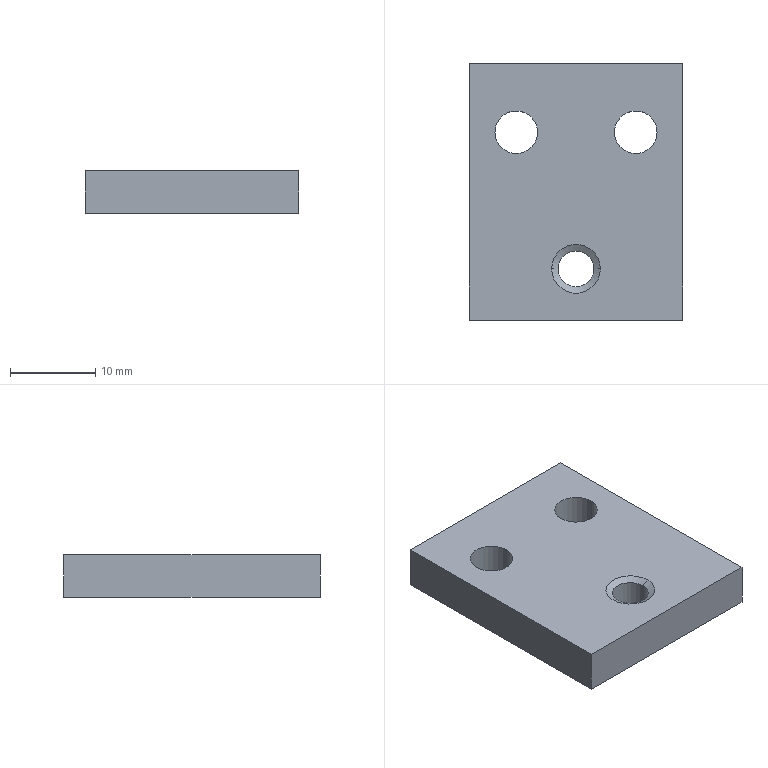Part | NX | 1 solid | 14 faces | box 25 x 30 x 5 mm | volume 3482 mm3 | plane 6 | cylinder 6 | cone 2 | commonest cylinder face diameters 5 x4 4.2 x2
STEP:
#1=CARTESIAN_POINT('',(-12.5,-9.53,2.5));
#2=VERTEX_POINT('',#1);
#3=CARTESIAN_POINT('',(-12.5,20.47,2.5));
#4=VERTEX_POINT('',#3);
#5=CARTESIAN_POINT('',(-12.5,0.,2.5));
#6=DIRECTION('',(0.,1.,0.));
#7=VECTOR('',#6,1000.);
#8=LINE('',#5,#7);
#9=EDGE_CURVE('',#2,#4,#8,.T.);
#10=ORIENTED_EDGE('',*,*,#9,.F.);
#11=CARTESIAN_POINT('',(12.5,-9.53,2.5));
#12=VERTEX_POINT('',#11);
#13=CARTESIAN_POINT('',(0.,-9.53,2.5));
#14=DIRECTION('',(-1.,0.,0.));
#15=VECTOR('',#14,1000.);
#16=LINE('',#13,#15);
#17=EDGE_CURVE('',#12,#2,#16,.T.);
#18=ORIENTED_EDGE('',*,*,#17,.F.);
#19=CARTESIAN_POINT('',(12.5,20.47,2.5));
#20=VERTEX_POINT('',#19);
#21=CARTESIAN_POINT('',(12.5,0.,2.5));
#22=DIRECTION('',(0.,1.,0.));
#23=VECTOR('',#22,1000.);
#24=LINE('',#21,#23);
#25=EDGE_CURVE('',#12,#20,#24,.T.);
#26=ORIENTED_EDGE('',*,*,#25,.T.);
#27=CARTESIAN_POINT('',(0.,20.47,2.5));
#28=DIRECTION('',(1.,0.,0.));
#29=VECTOR('',#28,1000.);
#30=LINE('',#27,#29);
#31=EDGE_CURVE('',#4,#20,#30,.T.);
#32=ORIENTED_EDGE('',*,*,#31,.F.);
#33=EDGE_LOOP('',(#10,#18,#26,#32));
#34=FACE_BOUND('',#33,.T.);
#35=CARTESIAN_POINT('',(-9.5,12.47,2.5));
#36=VERTEX_POINT('',#35);
#37=CARTESIAN_POINT('',(-4.5,12.47,2.5));
#38=VERTEX_POINT('',#37);
#39=CARTESIAN_POINT('',(-7.,12.47,2.5));
#40=DIRECTION('',(0.,0.,-1.));
#41=DIRECTION('',(-1.,0.,0.));
#42=AXIS2_PLACEMENT_3D('',#39,#40,#41);
#43=CIRCLE('',#42,2.5);
#44=EDGE_CURVE('',#36,#38,#43,.T.);
#45=ORIENTED_EDGE('',*,*,#44,.T.);
#46=CARTESIAN_POINT('',(-7.,12.47,2.5));
#47=DIRECTION('',(0.,0.,-1.));
#48=DIRECTION('',(-1.,0.,0.));
#49=AXIS2_PLACEMENT_3D('',#46,#47,#48);
#50=CIRCLE('',#49,2.5);
#51=EDGE_CURVE('',#38,#36,#50,.T.);
#52=ORIENTED_EDGE('',*,*,#51,.T.);
#53=EDGE_LOOP('',(#45,#52));
#54=FACE_BOUND('',#53,.T.);
#55=CARTESIAN_POINT('',(2.86,-3.53,2.5));
#56=VERTEX_POINT('',#55);
#57=CARTESIAN_POINT('',(-2.86,-3.53,2.5));
#58=VERTEX_POINT('',#57);
#59=CARTESIAN_POINT('',(0.,-3.53,2.5));
#60=DIRECTION('',(0.,0.,1.));
#61=DIRECTION('',(1.,0.,0.));
#62=AXIS2_PLACEMENT_3D('',#59,#60,#61);
#63=CIRCLE('',#62,2.86);
#64=EDGE_CURVE('',#56,#58,#63,.T.);
#65=ORIENTED_EDGE('',*,*,#64,.F.);
#66=CARTESIAN_POINT('',(0.,-3.53,2.5));
#67=DIRECTION('',(0.,0.,1.));
#68=DIRECTION('',(1.,0.,0.));
#69=AXIS2_PLACEMENT_3D('',#66,#67,#68);
#70=CIRCLE('',#69,2.86);
#71=EDGE_CURVE('',#58,#56,#70,.T.);
#72=ORIENTED_EDGE('',*,*,#71,.F.);
#73=EDGE_LOOP('',(#65,#72));
#74=FACE_BOUND('',#73,.T.);
#75=CARTESIAN_POINT('',(9.5,12.47,2.5));
#76=VERTEX_POINT('',#75);
#77=CARTESIAN_POINT('',(4.5,12.47,2.5));
#78=VERTEX_POINT('',#77);
#79=CARTESIAN_POINT('',(7.,12.47,2.5));
#80=DIRECTION('',(0.,0.,-1.));
#81=DIRECTION('',(-1.,0.,0.));
#82=AXIS2_PLACEMENT_3D('',#79,#80,#81);
#83=CIRCLE('',#82,2.5);
#84=EDGE_CURVE('',#76,#78,#83,.T.);
#85=ORIENTED_EDGE('',*,*,#84,.T.);
#86=CARTESIAN_POINT('',(7.,12.47,2.5));
#87=DIRECTION('',(0.,0.,-1.));
#88=DIRECTION('',(-1.,0.,0.));
#89=AXIS2_PLACEMENT_3D('',#86,#87,#88);
#90=CIRCLE('',#89,2.5);
#91=EDGE_CURVE('',#78,#76,#90,.T.);
#92=ORIENTED_EDGE('',*,*,#91,.T.);
#93=EDGE_LOOP('',(#85,#92));
#94=FACE_BOUND('',#93,.T.);
#95=CARTESIAN_POINT('',(0.,0.,2.5));
#96=DIRECTION('',(0.,0.,1.));
#97=DIRECTION('',(1.,0.,0.));
#98=AXIS2_PLACEMENT_3D('',#95,#96,#97);
#99=PLANE('',#98);
#100=ADVANCED_FACE('',(#34,#54,#74,#94),#99,.T.);
#101=CARTESIAN_POINT('',(-12.5,-9.53,-2.5));
#102=VERTEX_POINT('',#101);
#103=CARTESIAN_POINT('',(-12.5,20.47,-2.5));
#104=VERTEX_POINT('',#103);
#105=CARTESIAN_POINT('',(-12.5,0.,-2.5));
#106=DIRECTION('',(0.,1.,0.));
#107=VECTOR('',#106,1000.);
#108=LINE('',#105,#107);
#109=EDGE_CURVE('',#102,#104,#108,.T.);
#110=ORIENTED_EDGE('',*,*,#109,.F.);
#111=CARTESIAN_POINT('',(-12.5,-9.53,0.));
#112=DIRECTION('',(0.,0.,-1.));
#113=VECTOR('',#112,1000.);
#114=LINE('',#111,#113);
#115=EDGE_CURVE('',#2,#102,#114,.T.);
#116=ORIENTED_EDGE('',*,*,#115,.F.);
#117=ORIENTED_EDGE('',*,*,#9,.T.);
#118=CARTESIAN_POINT('',(-12.5,20.47,0.));
#119=DIRECTION('',(0.,0.,1.));
#120=VECTOR('',#119,1000.);
#121=LINE('',#118,#120);
#122=EDGE_CURVE('',#104,#4,#121,.T.);
#123=ORIENTED_EDGE('',*,*,#122,.F.);
#124=EDGE_LOOP('',(#110,#116,#117,#123));
#125=FACE_BOUND('',#124,.T.);
#126=CARTESIAN_POINT('',(-12.5,20.5,-2.5));
#127=DIRECTION('',(-1.,0.,0.));
#128=DIRECTION('',(0.,0.,1.));
#129=AXIS2_PLACEMENT_3D('',#126,#127,#128);
#130=PLANE('',#129);
#131=ADVANCED_FACE('',(#125),#130,.T.);
#132=CARTESIAN_POINT('',(12.5,20.47,-2.5));
#133=VERTEX_POINT('',#132);
#134=CARTESIAN_POINT('',(0.,20.47,-2.5));
#135=DIRECTION('',(1.,0.,0.));
#136=VECTOR('',#135,1000.);
#137=LINE('',#134,#136);
#138=EDGE_CURVE('',#104,#133,#137,.T.);
#139=ORIENTED_EDGE('',*,*,#138,.F.);
#140=ORIENTED_EDGE('',*,*,#122,.T.);
#141=ORIENTED_EDGE('',*,*,#31,.T.);
#142=CARTESIAN_POINT('',(12.5,20.47,0.));
#143=DIRECTION('',(0.,0.,-1.));
#144=VECTOR('',#143,1000.);
#145=LINE('',#142,#144);
#146=EDGE_CURVE('',#20,#133,#145,.T.);
#147=ORIENTED_EDGE('',*,*,#146,.T.);
#148=EDGE_LOOP('',(#139,#140,#141,#147));
#149=FACE_BOUND('',#148,.T.);
#150=CARTESIAN_POINT('',(-205.,20.47,-99.5));
#151=DIRECTION('',(0.,1.,0.));
#152=DIRECTION('',(1.,0.,0.));
#153=AXIS2_PLACEMENT_3D('',#150,#151,#152);
#154=PLANE('',#153);
#155=ADVANCED_FACE('',(#149),#154,.T.);
#156=ORIENTED_EDGE('',*,*,#64,.T.);
#157=CARTESIAN_POINT('',(-2.1,-3.53,2.061));
#158=VERTEX_POINT('',#157);
#159=CARTESIAN_POINT('',(-2.1,-3.53,2.061));
#160=DIRECTION('',(-0.866,0.,0.5));
#161=VECTOR('',#160,1000.);
#162=LINE('',#159,#161);
#163=EDGE_CURVE('',#158,#58,#162,.T.);
#164=ORIENTED_EDGE('',*,*,#163,.F.);
#165=CARTESIAN_POINT('',(2.1,-3.53,2.061));
#166=VERTEX_POINT('',#165);
#167=CARTESIAN_POINT('',(0.,-3.53,2.061));
#168=DIRECTION('',(0.,0.,1.));
#169=DIRECTION('',(1.,0.,0.));
#170=AXIS2_PLACEMENT_3D('',#167,#168,#169);
#171=CIRCLE('',#170,2.1);
#172=EDGE_CURVE('',#166,#158,#171,.T.);
#173=ORIENTED_EDGE('',*,*,#172,.F.);
#174=CARTESIAN_POINT('',(2.1,-3.53,2.061));
#175=DIRECTION('',(0.866,0.,0.5));
#176=VECTOR('',#175,1000.);
#177=LINE('',#174,#176);
#178=EDGE_CURVE('',#166,#56,#177,.T.);
#179=ORIENTED_EDGE('',*,*,#178,.T.);
#180=EDGE_LOOP('',(#156,#164,#173,#179));
#181=FACE_BOUND('',#180,.T.);
#182=CARTESIAN_POINT('',(0.,-3.53,2.061));
#183=DIRECTION('',(0.,0.,1.));
#184=DIRECTION('',(1.,0.,0.));
#185=AXIS2_PLACEMENT_3D('',#182,#183,#184);
#186=CONICAL_SURFACE('',#185,2.1,1.047);
#187=ADVANCED_FACE('',(#181),#186,.F.);
#188=CARTESIAN_POINT('',(12.5,-9.53,-2.5));
#189=VERTEX_POINT('',#188);
#190=CARTESIAN_POINT('',(12.5,-9.53,0.));
#191=DIRECTION('',(0.,0.,-1.));
#192=VECTOR('',#191,1000.);
#193=LINE('',#190,#192);
#194=EDGE_CURVE('',#12,#189,#193,.T.);
#195=ORIENTED_EDGE('',*,*,#194,.T.);
#196=CARTESIAN_POINT('',(12.5,0.,-2.5));
#197=DIRECTION('',(0.,-1.,0.));
#198=VECTOR('',#197,1000.);
#199=LINE('',#196,#198);
#200=EDGE_CURVE('',#133,#189,#199,.T.);
#201=ORIENTED_EDGE('',*,*,#200,.F.);
#202=ORIENTED_EDGE('',*,*,#146,.F.);
#203=ORIENTED_EDGE('',*,*,#25,.F.);
#204=EDGE_LOOP('',(#195,#201,#202,#203));
#205=FACE_BOUND('',#204,.T.);
#206=CARTESIAN_POINT('',(12.5,-20.5,-2.5));
#207=DIRECTION('',(1.,0.,0.));
#208=DIRECTION('',(0.,1.,0.));
#209=AXIS2_PLACEMENT_3D('',#206,#207,#208);
#210=PLANE('',#209);
#211=ADVANCED_FACE('',(#205),#210,.T.);
#212=ORIENTED_EDGE('',*,*,#109,.T.);
#213=ORIENTED_EDGE('',*,*,#138,.T.);
#214=ORIENTED_EDGE('',*,*,#200,.T.);
#215=CARTESIAN_POINT('',(0.,-9.53,-2.5));
#216=DIRECTION('',(1.,0.,0.));
#217=VECTOR('',#216,1000.);
#218=LINE('',#215,#217);
#219=EDGE_CURVE('',#102,#189,#218,.T.);
#220=ORIENTED_EDGE('',*,*,#219,.F.);
#221=EDGE_LOOP('',(#212,#213,#214,#220));
#222=FACE_BOUND('',#221,.T.);
#223=CARTESIAN_POINT('',(-9.5,12.47,-2.5));
#224=VERTEX_POINT('',#223);
#225=CARTESIAN_POINT('',(-4.5,12.47,-2.5));
#226=VERTEX_POINT('',#225);
#227=CARTESIAN_POINT('',(-7.,12.47,-2.5));
#228=DIRECTION('',(0.,0.,-1.));
#229=DIRECTION('',(-1.,0.,0.));
#230=AXIS2_PLACEMENT_3D('',#227,#228,#229);
#231=CIRCLE('',#230,2.5);
#232=EDGE_CURVE('',#224,#226,#231,.T.);
#233=ORIENTED_EDGE('',*,*,#232,.F.);
#234=CARTESIAN_POINT('',(-7.,12.47,-2.5));
#235=DIRECTION('',(0.,0.,-1.));
#236=DIRECTION('',(-1.,0.,0.));
#237=AXIS2_PLACEMENT_3D('',#234,#235,#236);
#238=CIRCLE('',#237,2.5);
#239=EDGE_CURVE('',#226,#224,#238,.T.);
#240=ORIENTED_EDGE('',*,*,#239,.F.);
#241=EDGE_LOOP('',(#233,#240));
#242=FACE_BOUND('',#241,.T.);
#243=CARTESIAN_POINT('',(9.5,12.47,-2.5));
#244=VERTEX_POINT('',#243);
#245=CARTESIAN_POINT('',(4.5,12.47,-2.5));
#246=VERTEX_POINT('',#245);
#247=CARTESIAN_POINT('',(7.,12.47,-2.5));
#248=DIRECTION('',(0.,0.,-1.));
#249=DIRECTION('',(-1.,0.,0.));
#250=AXIS2_PLACEMENT_3D('',#247,#248,#249);
#251=CIRCLE('',#250,2.5);
#252=EDGE_CURVE('',#244,#246,#251,.T.);
#253=ORIENTED_EDGE('',*,*,#252,.F.);
#254=CARTESIAN_POINT('',(7.,12.47,-2.5));
#255=DIRECTION('',(0.,0.,-1.));
#256=DIRECTION('',(-1.,0.,0.));
#257=AXIS2_PLACEMENT_3D('',#254,#255,#256);
#258=CIRCLE('',#257,2.5);
#259=EDGE_CURVE('',#246,#244,#258,.T.);
#260=ORIENTED_EDGE('',*,*,#259,.F.);
#261=EDGE_LOOP('',(#253,#260));
#262=FACE_BOUND('',#261,.T.);
#263=CARTESIAN_POINT('',(-2.1,-3.53,-2.5));
#264=VERTEX_POINT('',#263);
#265=CARTESIAN_POINT('',(2.1,-3.53,-2.5));
#266=VERTEX_POINT('',#265);
#267=CARTESIAN_POINT('',(0.,-3.53,-2.5));
#268=DIRECTION('',(0.,0.,1.));
#269=DIRECTION('',(1.,0.,0.));
#270=AXIS2_PLACEMENT_3D('',#267,#268,#269);
#271=CIRCLE('',#270,2.1);
#272=EDGE_CURVE('',#264,#266,#271,.T.);
#273=ORIENTED_EDGE('',*,*,#272,.T.);
#274=CARTESIAN_POINT('',(0.,-3.53,-2.5));
#275=DIRECTION('',(0.,0.,1.));
#276=DIRECTION('',(1.,0.,0.));
#277=AXIS2_PLACEMENT_3D('',#274,#275,#276);
#278=CIRCLE('',#277,2.1);
#279=EDGE_CURVE('',#266,#264,#278,.T.);
#280=ORIENTED_EDGE('',*,*,#279,.T.);
#281=EDGE_LOOP('',(#273,#280));
#282=FACE_BOUND('',#281,.T.);
#283=CARTESIAN_POINT('',(0.,0.,-2.5));
#284=DIRECTION('',(0.,0.,1.));
#285=DIRECTION('',(1.,0.,0.));
#286=AXIS2_PLACEMENT_3D('',#283,#284,#285);
#287=PLANE('',#286);
#288=ADVANCED_FACE('',(#222,#242,#262,#282),#287,.F.);
#289=ORIENTED_EDGE('',*,*,#232,.T.);
#290=CARTESIAN_POINT('',(-4.5,12.47,2.5));
#291=DIRECTION('',(0.,0.,-1.));
#292=VECTOR('',#291,1000.);
#293=LINE('',#290,#292);
#294=EDGE_CURVE('',#226,#38,#293,.F.);
#295=ORIENTED_EDGE('',*,*,#294,.T.);
#296=ORIENTED_EDGE('',*,*,#44,.F.);
#297=CARTESIAN_POINT('',(-9.5,12.47,2.5));
#298=DIRECTION('',(0.,0.,-1.));
#299=VECTOR('',#298,1000.);
#300=LINE('',#297,#299);
#301=EDGE_CURVE('',#224,#36,#300,.F.);
#302=ORIENTED_EDGE('',*,*,#301,.F.);
#303=EDGE_LOOP('',(#289,#295,#296,#302));
#304=FACE_BOUND('',#303,.T.);
#305=CARTESIAN_POINT('',(-7.,12.47,2.5));
#306=DIRECTION('',(0.,0.,-1.));
#307=DIRECTION('',(-1.,0.,0.));
#308=AXIS2_PLACEMENT_3D('',#305,#306,#307);
#309=CYLINDRICAL_SURFACE('',#308,2.5);
#310=ADVANCED_FACE('',(#304),#309,.F.);
#311=ORIENTED_EDGE('',*,*,#252,.T.);
#312=CARTESIAN_POINT('',(4.5,12.47,2.5));
#313=DIRECTION('',(0.,0.,-1.));
#314=VECTOR('',#313,1000.);
#315=LINE('',#312,#314);
#316=EDGE_CURVE('',#246,#78,#315,.F.);
#317=ORIENTED_EDGE('',*,*,#316,.T.);
#318=ORIENTED_EDGE('',*,*,#84,.F.);
#319=CARTESIAN_POINT('',(9.5,12.47,2.5));
#320=DIRECTION('',(0.,0.,-1.));
#321=VECTOR('',#320,1000.);
#322=LINE('',#319,#321);
#323=EDGE_CURVE('',#244,#76,#322,.F.);
#324=ORIENTED_EDGE('',*,*,#323,.F.);
#325=EDGE_LOOP('',(#311,#317,#318,#324));
#326=FACE_BOUND('',#325,.T.);
#327=CARTESIAN_POINT('',(7.,12.47,2.5));
#328=DIRECTION('',(0.,0.,-1.));
#329=DIRECTION('',(-1.,0.,0.));
#330=AXIS2_PLACEMENT_3D('',#327,#328,#329);
#331=CYLINDRICAL_SURFACE('',#330,2.5);
#332=ADVANCED_FACE('',(#326),#331,.F.);
#333=ORIENTED_EDGE('',*,*,#172,.T.);
#334=CARTESIAN_POINT('',(-2.1,-3.53,2.5));
#335=DIRECTION('',(0.,0.,1.));
#336=VECTOR('',#335,1000.);
#337=LINE('',#334,#336);
#338=EDGE_CURVE('',#158,#264,#337,.F.);
#339=ORIENTED_EDGE('',*,*,#338,.T.);
#340=ORIENTED_EDGE('',*,*,#279,.F.);
#341=CARTESIAN_POINT('',(2.1,-3.53,2.5));
#342=DIRECTION('',(0.,0.,1.));
#343=VECTOR('',#342,1000.);
#344=LINE('',#341,#343);
#345=EDGE_CURVE('',#166,#266,#344,.F.);
#346=ORIENTED_EDGE('',*,*,#345,.F.);
#347=EDGE_LOOP('',(#333,#339,#340,#346));
#348=FACE_BOUND('',#347,.T.);
#349=CARTESIAN_POINT('',(0.,-3.53,2.5));
#350=DIRECTION('',(0.,0.,1.));
#351=DIRECTION('',(1.,0.,0.));
#352=AXIS2_PLACEMENT_3D('',#349,#350,#351);
#353=CYLINDRICAL_SURFACE('',#352,2.1);
#354=ADVANCED_FACE('',(#348),#353,.F.);
#355=ORIENTED_EDGE('',*,*,#219,.T.);
#356=ORIENTED_EDGE('',*,*,#194,.F.);
#357=ORIENTED_EDGE('',*,*,#17,.T.);
#358=ORIENTED_EDGE('',*,*,#115,.T.);
#359=EDGE_LOOP('',(#355,#356,#357,#358));
#360=FACE_BOUND('',#359,.T.);
#361=CARTESIAN_POINT('',(12.5,-9.53,3.));
#362=DIRECTION('',(0.,1.,0.));
#363=DIRECTION('',(1.,0.,0.));
#364=AXIS2_PLACEMENT_3D('',#361,#362,#363);
#365=PLANE('',#364);
#366=ADVANCED_FACE('',(#360),#365,.F.);
#367=ORIENTED_EDGE('',*,*,#316,.F.);
#368=ORIENTED_EDGE('',*,*,#259,.T.);
#369=ORIENTED_EDGE('',*,*,#323,.T.);
#370=ORIENTED_EDGE('',*,*,#91,.F.);
#371=EDGE_LOOP('',(#367,#368,#369,#370));
#372=FACE_BOUND('',#371,.T.);
#373=CARTESIAN_POINT('',(7.,12.47,2.5));
#374=DIRECTION('',(0.,0.,-1.));
#375=DIRECTION('',(-1.,0.,0.));
#376=AXIS2_PLACEMENT_3D('',#373,#374,#375);
#377=CYLINDRICAL_SURFACE('',#376,2.5);
#378=ADVANCED_FACE('',(#372),#377,.F.);
#379=ORIENTED_EDGE('',*,*,#301,.T.);
#380=ORIENTED_EDGE('',*,*,#51,.F.);
#381=ORIENTED_EDGE('',*,*,#294,.F.);
#382=ORIENTED_EDGE('',*,*,#239,.T.);
#383=EDGE_LOOP('',(#379,#380,#381,#382));
#384=FACE_BOUND('',#383,.T.);
#385=CARTESIAN_POINT('',(-7.,12.47,2.5));
#386=DIRECTION('',(0.,0.,-1.));
#387=DIRECTION('',(-1.,0.,0.));
#388=AXIS2_PLACEMENT_3D('',#385,#386,#387);
#389=CYLINDRICAL_SURFACE('',#388,2.5);
#390=ADVANCED_FACE('',(#384),#389,.F.);
#391=ORIENTED_EDGE('',*,*,#178,.F.);
#392=CARTESIAN_POINT('',(0.,-3.53,2.061));
#393=DIRECTION('',(0.,0.,1.));
#394=DIRECTION('',(1.,0.,0.));
#395=AXIS2_PLACEMENT_3D('',#392,#393,#394);
#396=CIRCLE('',#395,2.1);
#397=EDGE_CURVE('',#158,#166,#396,.T.);
#398=ORIENTED_EDGE('',*,*,#397,.F.);
#399=ORIENTED_EDGE('',*,*,#163,.T.);
#400=ORIENTED_EDGE('',*,*,#71,.T.);
#401=EDGE_LOOP('',(#391,#398,#399,#400));
#402=FACE_BOUND('',#401,.T.);
#403=CARTESIAN_POINT('',(0.,-3.53,2.061));
#404=DIRECTION('',(0.,0.,1.));
#405=DIRECTION('',(1.,0.,0.));
#406=AXIS2_PLACEMENT_3D('',#403,#404,#405);
#407=CONICAL_SURFACE('',#406,2.1,1.047);
#408=ADVANCED_FACE('',(#402),#407,.F.);
#409=ORIENTED_EDGE('',*,*,#272,.F.);
#410=ORIENTED_EDGE('',*,*,#338,.F.);
#411=ORIENTED_EDGE('',*,*,#397,.T.);
#412=ORIENTED_EDGE('',*,*,#345,.T.);
#413=EDGE_LOOP('',(#409,#410,#411,#412));
#414=FACE_BOUND('',#413,.T.);
#415=CARTESIAN_POINT('',(0.,-3.53,2.5));
#416=DIRECTION('',(0.,0.,1.));
#417=DIRECTION('',(1.,0.,0.));
#418=AXIS2_PLACEMENT_3D('',#415,#416,#417);
#419=CYLINDRICAL_SURFACE('',#418,2.1);
#420=ADVANCED_FACE('',(#414),#419,.F.);
#421=CLOSED_SHELL('',(#100,#131,#155,#187,#211,#288,#310,#332,#354,#366,#378,#390,#408,#420));
#422=MANIFOLD_SOLID_BREP('',#421);
#423=(LENGTH_UNIT()NAMED_UNIT(*)SI_UNIT(.MILLI.,.METRE.));
#424=UNCERTAINTY_MEASURE_WITH_UNIT(LENGTH_MEASURE(0.00001),#423,'','');
#425=(NAMED_UNIT(*)PLANE_ANGLE_UNIT()SI_UNIT($,.RADIAN.));
#426=(NAMED_UNIT(*)SI_UNIT($,.STERADIAN.)SOLID_ANGLE_UNIT());
#427=(GEOMETRIC_REPRESENTATION_CONTEXT(3)GLOBAL_UNCERTAINTY_ASSIGNED_CONTEXT((#424))GLOBAL_UNIT_ASSIGNED_CONTEXT((#423,#425,#426))REPRESENTATION_CONTEXT('',''));
#428=ADVANCED_BREP_SHAPE_REPRESENTATION('',(#422),#427);